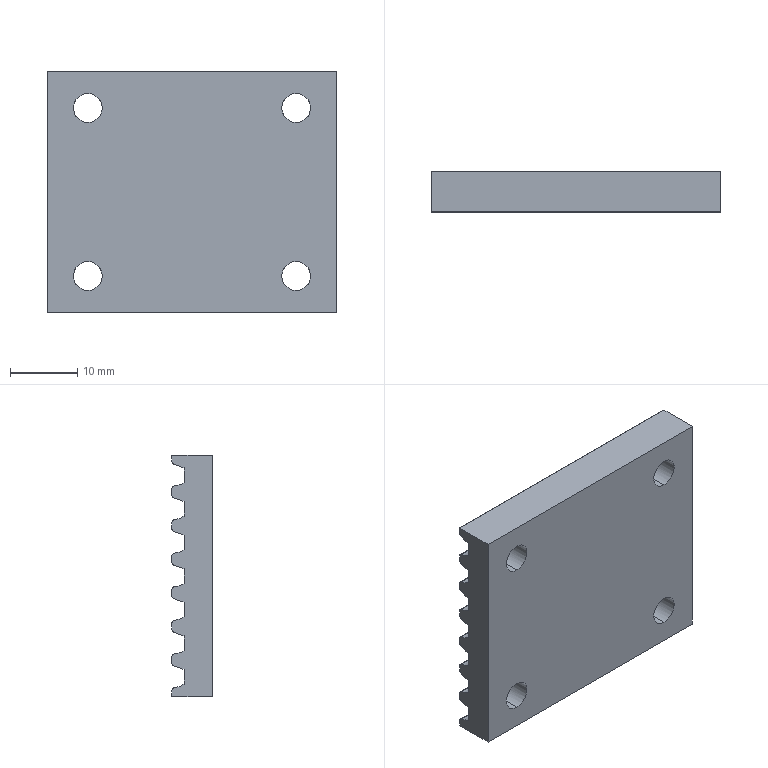Part | SolidWorks | features BaseBody 1 | 1 solid | 78 faces | box 43 x 6 x 36 mm | volume 7398 mm3 | cylinder 43 | plane 35 | commonest cylinder face diameters 1 x24 6.522 x11 4.3 x8